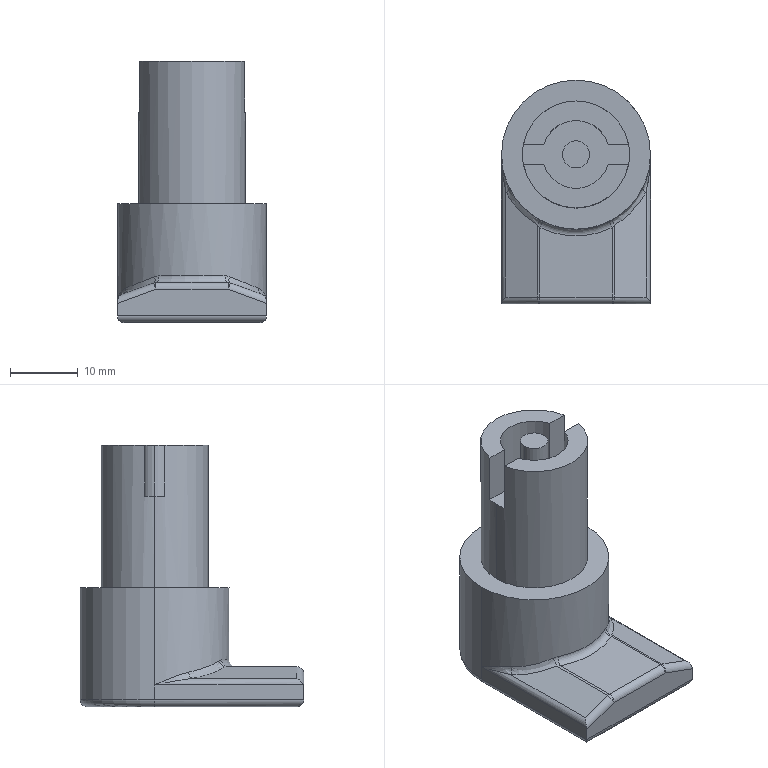Part | STEP file | 1 solid | 67 faces | box 22 x 33 x 38.56 mm | volume 10259 mm3 | plane 37 | cylinder 20 | spline 6 | torus 2 | sphere 2 | commonest cylinder face diameters 2 x10 4 x2 10 x2 15 x2 15.8 x2 22 x2